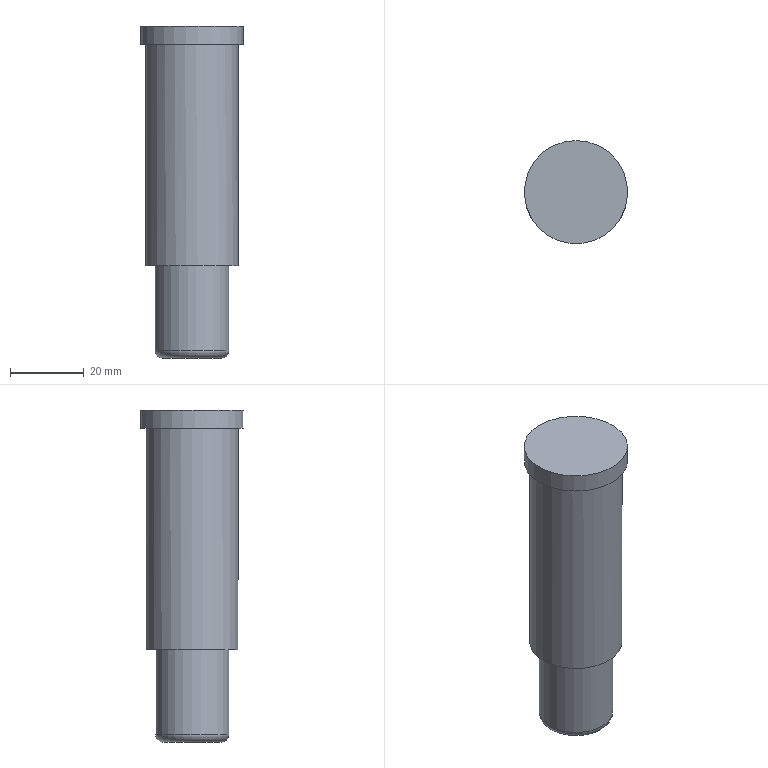Part | NX | features MAIN_BODY 2 | 1 solid | 8 faces | box 28 x 28 x 90 mm | volume 40334 mm3 | plane 4 | cylinder 3 | torus 1 | commonest cylinder face diameters 20 x1 25 x1 28 x1
STEP:
#1=CARTESIAN_POINT('',(422.506,28.27,53.));
#2=VERTEX_POINT('',#1);
#3=CARTESIAN_POINT('',(435.006,28.27,53.));
#4=DIRECTION('',(0.,0.,-1.));
#5=DIRECTION('',(-1.,0.,0.));
#6=AXIS2_PLACEMENT_3D('',#3,#4,#5);
#7=CIRCLE('',#6,12.5);
#8=EDGE_CURVE('',#2,#2,#7,.T.);
#9=ORIENTED_EDGE('',*,*,#8,.F.);
#10=EDGE_LOOP('',(#9));
#11=FACE_BOUND('',#10,.T.);
#12=CARTESIAN_POINT('',(447.316,30.441,113.));
#13=VERTEX_POINT('',#12);
#14=CARTESIAN_POINT('',(435.006,28.27,113.));
#15=DIRECTION('',(0.,0.,-1.));
#16=DIRECTION('',(0.9848,0.1736,0.));
#17=AXIS2_PLACEMENT_3D('',#14,#15,#16);
#18=CIRCLE('',#17,12.5);
#19=EDGE_CURVE('',#13,#13,#18,.T.);
#20=ORIENTED_EDGE('',*,*,#19,.T.);
#21=EDGE_LOOP('',(#20));
#22=FACE_BOUND('',#21,.T.);
#23=CARTESIAN_POINT('',(435.006,28.27,118.));
#24=DIRECTION('',(0.,0.,-1.));
#25=DIRECTION('',(-0.9848,-0.1736,0.));
#26=AXIS2_PLACEMENT_3D('',#23,#24,#25);
#27=CYLINDRICAL_SURFACE('',#26,12.5);
#28=ADVANCED_FACE('',(#11,#22),#27,.T.);
#29=CARTESIAN_POINT('',(425.006,28.27,53.));
#30=VERTEX_POINT('',#29);
#31=CARTESIAN_POINT('',(435.006,28.27,53.));
#32=DIRECTION('',(0.,0.,-1.));
#33=DIRECTION('',(-1.,0.,0.));
#34=AXIS2_PLACEMENT_3D('',#31,#32,#33);
#35=CIRCLE('',#34,10.);
#36=EDGE_CURVE('',#30,#30,#35,.T.);
#37=ORIENTED_EDGE('',*,*,#36,.F.);
#38=EDGE_LOOP('',(#37));
#39=FACE_BOUND('',#38,.T.);
#40=ORIENTED_EDGE('',*,*,#8,.T.);
#41=EDGE_LOOP('',(#40));
#42=FACE_BOUND('',#41,.T.);
#43=CARTESIAN_POINT('',(435.006,28.27,53.));
#44=DIRECTION('',(0.,0.,1.));
#45=DIRECTION('',(0.9848,0.1736,0.));
#46=AXIS2_PLACEMENT_3D('',#43,#44,#45);
#47=PLANE('',#46);
#48=ADVANCED_FACE('',(#39,#42),#47,.F.);
#49=CARTESIAN_POINT('',(448.793,30.701,113.));
#50=VERTEX_POINT('',#49);
#51=CARTESIAN_POINT('',(435.006,28.27,113.));
#52=DIRECTION('',(0.,0.,-1.));
#53=DIRECTION('',(0.9848,0.1736,0.));
#54=AXIS2_PLACEMENT_3D('',#51,#52,#53);
#55=CIRCLE('',#54,14.);
#56=EDGE_CURVE('',#50,#50,#55,.T.);
#57=ORIENTED_EDGE('',*,*,#56,.T.);
#58=EDGE_LOOP('',(#57));
#59=FACE_BOUND('',#58,.T.);
#60=ORIENTED_EDGE('',*,*,#19,.F.);
#61=EDGE_LOOP('',(#60));
#62=FACE_BOUND('',#61,.T.);
#63=CARTESIAN_POINT('',(435.006,28.27,113.));
#64=DIRECTION('',(0.,0.,1.));
#65=DIRECTION('',(0.9848,0.1736,0.));
#66=AXIS2_PLACEMENT_3D('',#63,#64,#65);
#67=PLANE('',#66);
#68=ADVANCED_FACE('',(#59,#62),#67,.F.);
#69=ORIENTED_EDGE('',*,*,#56,.F.);
#70=EDGE_LOOP('',(#69));
#71=FACE_BOUND('',#70,.T.);
#72=CARTESIAN_POINT('',(448.793,30.701,118.));
#73=VERTEX_POINT('',#72);
#74=CARTESIAN_POINT('',(435.006,28.27,118.));
#75=DIRECTION('',(0.,0.,-1.));
#76=DIRECTION('',(0.9848,0.1736,0.));
#77=AXIS2_PLACEMENT_3D('',#74,#75,#76);
#78=CIRCLE('',#77,14.);
#79=EDGE_CURVE('',#73,#73,#78,.T.);
#80=ORIENTED_EDGE('',*,*,#79,.T.);
#81=EDGE_LOOP('',(#80));
#82=FACE_BOUND('',#81,.T.);
#83=CARTESIAN_POINT('',(435.006,28.27,114.));
#84=DIRECTION('',(0.,0.,1.));
#85=DIRECTION('',(0.9848,0.1736,0.));
#86=AXIS2_PLACEMENT_3D('',#83,#84,#85);
#87=CYLINDRICAL_SURFACE('',#86,14.);
#88=ADVANCED_FACE('',(#71,#82),#87,.T.);
#89=ORIENTED_EDGE('',*,*,#79,.F.);
#90=EDGE_LOOP('',(#89));
#91=FACE_BOUND('',#90,.T.);
#92=CARTESIAN_POINT('',(435.006,28.27,118.));
#93=DIRECTION('',(0.,0.,1.));
#94=DIRECTION('',(0.9848,0.1736,0.));
#95=AXIS2_PLACEMENT_3D('',#92,#93,#94);
#96=PLANE('',#95);
#97=ADVANCED_FACE('',(#91),#96,.T.);
#98=CARTESIAN_POINT('',(425.006,28.27,30.));
#99=VERTEX_POINT('',#98);
#100=CARTESIAN_POINT('',(435.006,28.27,30.));
#101=DIRECTION('',(0.,0.,-1.));
#102=DIRECTION('',(-1.,0.,0.));
#103=AXIS2_PLACEMENT_3D('',#100,#101,#102);
#104=CIRCLE('',#103,10.);
#105=EDGE_CURVE('',#99,#99,#104,.T.);
#106=ORIENTED_EDGE('',*,*,#105,.F.);
#107=EDGE_LOOP('',(#106));
#108=FACE_BOUND('',#107,.T.);
#109=ORIENTED_EDGE('',*,*,#36,.T.);
#110=EDGE_LOOP('',(#109));
#111=FACE_BOUND('',#110,.T.);
#112=CARTESIAN_POINT('',(435.006,28.27,38.));
#113=DIRECTION('',(0.,0.,1.));
#114=DIRECTION('',(0.9848,0.1736,0.));
#115=AXIS2_PLACEMENT_3D('',#112,#113,#114);
#116=CYLINDRICAL_SURFACE('',#115,10.);
#117=ADVANCED_FACE('',(#108,#111),#116,.T.);
#118=CARTESIAN_POINT('',(427.006,28.27,28.));
#119=VERTEX_POINT('',#118);
#120=CARTESIAN_POINT('',(435.006,28.27,28.));
#121=DIRECTION('',(0.,0.,-1.));
#122=DIRECTION('',(-1.,0.,0.));
#123=AXIS2_PLACEMENT_3D('',#120,#121,#122);
#124=CIRCLE('',#123,8.);
#125=EDGE_CURVE('',#119,#119,#124,.F.);
#126=ORIENTED_EDGE('',*,*,#125,.F.);
#127=EDGE_LOOP('',(#126));
#128=FACE_BOUND('',#127,.T.);
#129=CARTESIAN_POINT('',(435.006,28.27,28.));
#130=DIRECTION('',(0.,0.,1.));
#131=DIRECTION('',(0.9848,0.1736,0.));
#132=AXIS2_PLACEMENT_3D('',#129,#130,#131);
#133=PLANE('',#132);
#134=ADVANCED_FACE('',(#128),#133,.F.);
#135=ORIENTED_EDGE('',*,*,#125,.T.);
#136=EDGE_LOOP('',(#135));
#137=FACE_BOUND('',#136,.T.);
#138=ORIENTED_EDGE('',*,*,#105,.T.);
#139=EDGE_LOOP('',(#138));
#140=FACE_BOUND('',#139,.T.);
#141=CARTESIAN_POINT('',(435.006,28.27,30.));
#142=DIRECTION('',(0.,0.,1.));
#143=DIRECTION('',(-1.,0.,0.));
#144=AXIS2_PLACEMENT_3D('',#141,#142,#143);
#145=TOROIDAL_SURFACE('',#144,8.,2.);
#146=ADVANCED_FACE('',(#137,#140),#145,.T.);
#147=CLOSED_SHELL('',(#28,#48,#68,#88,#97,#117,#134,#146));
#148=MANIFOLD_SOLID_BREP('',#147);
#149=(LENGTH_UNIT()NAMED_UNIT(*)SI_UNIT(.MILLI.,.METRE.));
#150=UNCERTAINTY_MEASURE_WITH_UNIT(LENGTH_MEASURE(0.00001),#149,'','');
#151=(NAMED_UNIT(*)PLANE_ANGLE_UNIT()SI_UNIT($,.RADIAN.));
#152=(NAMED_UNIT(*)SI_UNIT($,.STERADIAN.)SOLID_ANGLE_UNIT());
#153=(GEOMETRIC_REPRESENTATION_CONTEXT(3)GLOBAL_UNCERTAINTY_ASSIGNED_CONTEXT((#150))GLOBAL_UNIT_ASSIGNED_CONTEXT((#149,#151,#152))REPRESENTATION_CONTEXT('',''));
#154=ADVANCED_BREP_SHAPE_REPRESENTATION('',(#148),#153);